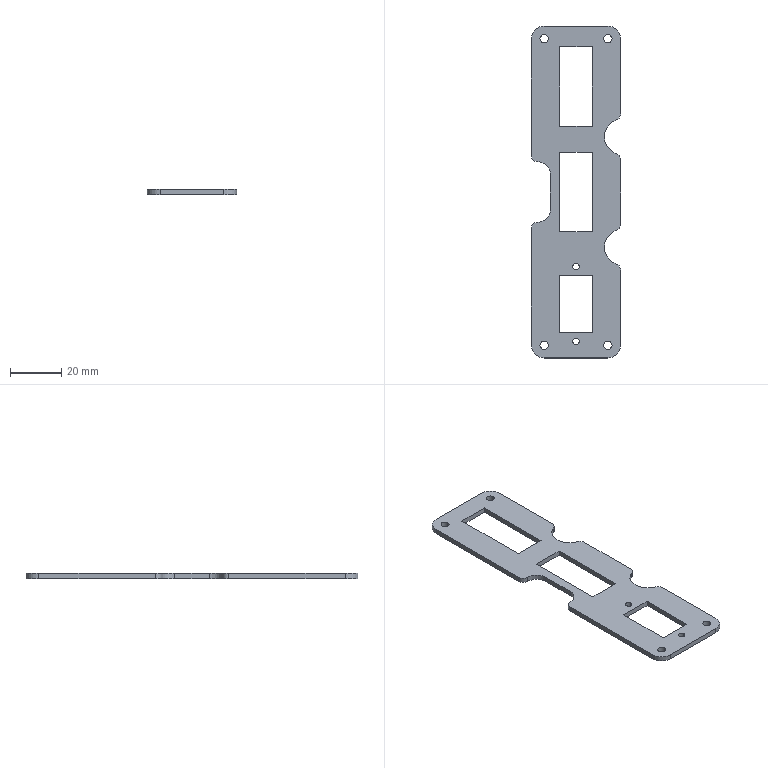Part | NX | features BREP 1 | 1 solid | 48 faces | box 35 x 130 x 2 mm | volume 6211 mm3 | cylinder 26 | plane 22 | commonest cylinder face diameters 3.2 x8 5 x6 10 x6 2.5 x4 14 x2